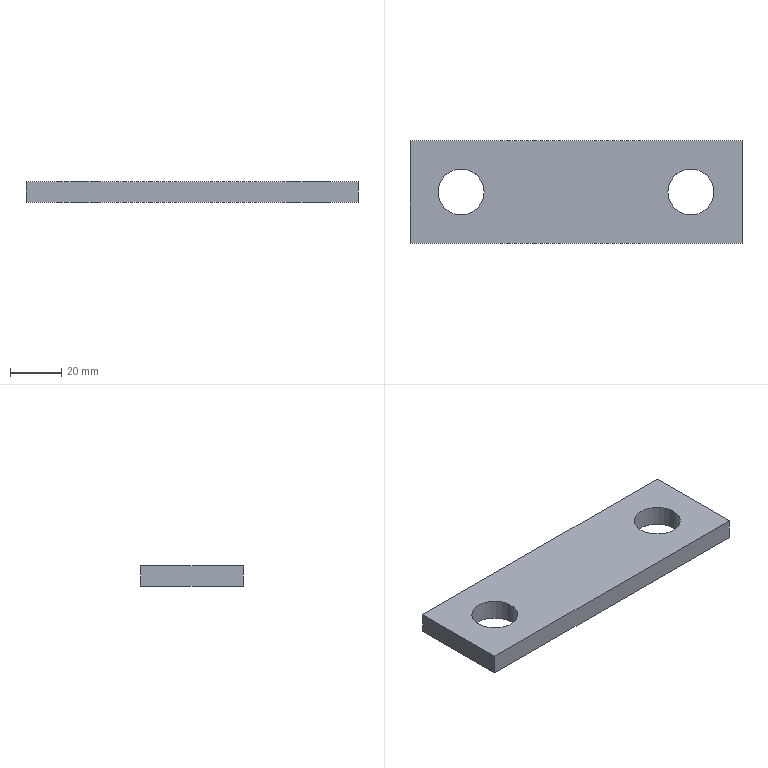Part | STEP file | JBZQ4348-1997 shaft end baffle 60 | 1 solid | 10 faces | box 130 x 40 x 8 mm | volume 37528 mm3 | plane 6 | cylinder 4 | commonest cylinder face diameters 18 x4
STEP:
#1=CARTESIAN_POINT('',(0.,0.,0.));
#2=DIRECTION('',(0.,0.,1.));
#3=DIRECTION('',(1.,0.,0.));
#4=AXIS2_PLACEMENT_3D('',#1,#2,#3);
#5=CARTESIAN_POINT('',(36.,0.,8.));
#6=VERTEX_POINT('',#5);
#7=CARTESIAN_POINT('',(36.,0.,0.));
#8=VERTEX_POINT('',#7);
#9=CARTESIAN_POINT('',(36.,0.,8.));
#10=DIRECTION('',(0.,0.,-1.));
#11=VECTOR('',#10,1.);
#12=LINE('',#9,#11);
#13=CARTESIAN_POINT('',(45.,0.,8.));
#14=DIRECTION('',(0.,0.,-1.));
#15=DIRECTION('',(-1.,0.,0.));
#16=AXIS2_PLACEMENT_3D('',#13,#14,#15);
#17=CYLINDRICAL_SURFACE('',#16,9.);
#18=CARTESIAN_POINT('',(6.283,0.));
#19=DIRECTION('',(0.,1.));
#20=VECTOR('',#19,1.);
#21=LINE('',#18,#20);
#22=(GEOMETRIC_REPRESENTATION_CONTEXT(2)PARAMETRIC_REPRESENTATION_CONTEXT()REPRESENTATION_CONTEXT('',''));
#23=DEFINITIONAL_REPRESENTATION('',(#21),#22);
#24=PCURVE('',#17,#23);
#25=CARTESIAN_POINT('',(45.,0.,8.));
#26=DIRECTION('',(0.,0.,-1.));
#27=DIRECTION('',(-1.,0.,0.));
#28=AXIS2_PLACEMENT_3D('',#25,#26,#27);
#29=CYLINDRICAL_SURFACE('',#28,9.);
#30=CARTESIAN_POINT('',(0.,0.));
#31=DIRECTION('',(0.,1.));
#32=VECTOR('',#31,1.);
#33=LINE('',#30,#32);
#34=(GEOMETRIC_REPRESENTATION_CONTEXT(2)PARAMETRIC_REPRESENTATION_CONTEXT()REPRESENTATION_CONTEXT('',''));
#35=DEFINITIONAL_REPRESENTATION('',(#33),#34);
#36=PCURVE('',#29,#35);
#37=SURFACE_CURVE('',#12,(#24,#36),.PCURVE_S1.);
#38=EDGE_CURVE('',#6,#8,#37,.T.);
#39=ORIENTED_EDGE('',*,*,#38,.T.);
#40=CARTESIAN_POINT('',(54.,0.,0.));
#41=VERTEX_POINT('',#40);
#42=CARTESIAN_POINT('',(45.,0.,0.));
#43=DIRECTION('',(0.,0.,1.));
#44=DIRECTION('',(1.,0.,0.));
#45=AXIS2_PLACEMENT_3D('',#42,#43,#44);
#46=CIRCLE('',#45,9.);
#47=CARTESIAN_POINT('',(9.425,8.));
#48=DIRECTION('',(-1.,0.));
#49=VECTOR('',#48,1.);
#50=LINE('',#47,#49);
#51=(GEOMETRIC_REPRESENTATION_CONTEXT(2)PARAMETRIC_REPRESENTATION_CONTEXT()REPRESENTATION_CONTEXT('',''));
#52=DEFINITIONAL_REPRESENTATION('',(#50),#51);
#53=PCURVE('',#17,#52);
#54=CARTESIAN_POINT('',(-65.,20.,0.));
#55=DIRECTION('',(0.,0.,1.));
#56=DIRECTION('',(1.,0.,0.));
#57=AXIS2_PLACEMENT_3D('',#54,#55,#56);
#58=PLANE('',#57);
#59=CARTESIAN_POINT('',(110.,-20.));
#60=DIRECTION('',(1.,0.));
#61=AXIS2_PLACEMENT_2D('',#59,#60);
#62=CIRCLE('',#61,9.);
#63=(GEOMETRIC_REPRESENTATION_CONTEXT(2)PARAMETRIC_REPRESENTATION_CONTEXT()REPRESENTATION_CONTEXT('',''));
#64=DEFINITIONAL_REPRESENTATION('',(#62),#63);
#65=PCURVE('',#58,#64);
#66=SURFACE_CURVE('',#46,(#53,#65),.PCURVE_S1.);
#67=EDGE_CURVE('',#8,#41,#66,.T.);
#68=ORIENTED_EDGE('',*,*,#67,.T.);
#69=CARTESIAN_POINT('',(54.,0.,8.));
#70=VERTEX_POINT('',#69);
#71=CARTESIAN_POINT('',(54.,0.,8.));
#72=DIRECTION('',(0.,0.,-1.));
#73=VECTOR('',#72,1.);
#74=LINE('',#71,#73);
#75=CARTESIAN_POINT('',(3.142,0.));
#76=DIRECTION('',(0.,1.));
#77=VECTOR('',#76,1.);
#78=LINE('',#75,#77);
#79=(GEOMETRIC_REPRESENTATION_CONTEXT(2)PARAMETRIC_REPRESENTATION_CONTEXT()REPRESENTATION_CONTEXT('',''));
#80=DEFINITIONAL_REPRESENTATION('',(#78),#79);
#81=PCURVE('',#17,#80);
#82=CARTESIAN_POINT('',(3.142,0.));
#83=DIRECTION('',(0.,1.));
#84=VECTOR('',#83,1.);
#85=LINE('',#82,#84);
#86=(GEOMETRIC_REPRESENTATION_CONTEXT(2)PARAMETRIC_REPRESENTATION_CONTEXT()REPRESENTATION_CONTEXT('',''));
#87=DEFINITIONAL_REPRESENTATION('',(#85),#86);
#88=PCURVE('',#29,#87);
#89=SURFACE_CURVE('',#74,(#81,#88),.PCURVE_S1.);
#90=EDGE_CURVE('',#70,#41,#89,.T.);
#91=ORIENTED_EDGE('',*,*,#90,.F.);
#92=CARTESIAN_POINT('',(45.,0.,8.));
#93=DIRECTION('',(0.,0.,1.));
#94=DIRECTION('',(1.,0.,0.));
#95=AXIS2_PLACEMENT_3D('',#92,#93,#94);
#96=CIRCLE('',#95,9.);
#97=CARTESIAN_POINT('',(9.425,0.));
#98=DIRECTION('',(-1.,0.));
#99=VECTOR('',#98,1.);
#100=LINE('',#97,#99);
#101=(GEOMETRIC_REPRESENTATION_CONTEXT(2)PARAMETRIC_REPRESENTATION_CONTEXT()REPRESENTATION_CONTEXT('',''));
#102=DEFINITIONAL_REPRESENTATION('',(#100),#101);
#103=PCURVE('',#17,#102);
#104=CARTESIAN_POINT('',(-65.,20.,8.));
#105=DIRECTION('',(0.,0.,1.));
#106=DIRECTION('',(1.,0.,0.));
#107=AXIS2_PLACEMENT_3D('',#104,#105,#106);
#108=PLANE('',#107);
#109=CARTESIAN_POINT('',(110.,-20.));
#110=DIRECTION('',(1.,0.));
#111=AXIS2_PLACEMENT_2D('',#109,#110);
#112=CIRCLE('',#111,9.);
#113=(GEOMETRIC_REPRESENTATION_CONTEXT(2)PARAMETRIC_REPRESENTATION_CONTEXT()REPRESENTATION_CONTEXT('',''));
#114=DEFINITIONAL_REPRESENTATION('',(#112),#113);
#115=PCURVE('',#108,#114);
#116=SURFACE_CURVE('',#96,(#103,#115),.PCURVE_S1.);
#117=EDGE_CURVE('',#6,#70,#116,.T.);
#118=ORIENTED_EDGE('',*,*,#117,.F.);
#119=EDGE_LOOP('',(#39,#68,#91,#118));
#120=FACE_BOUND('',#119,.F.);
#121=ADVANCED_FACE('',(#120),#17,.F.);
#122=CARTESIAN_POINT('',(-54.,0.,8.));
#123=VERTEX_POINT('',#122);
#124=CARTESIAN_POINT('',(-54.,0.,0.));
#125=VERTEX_POINT('',#124);
#126=CARTESIAN_POINT('',(-54.,0.,8.));
#127=DIRECTION('',(0.,0.,-1.));
#128=VECTOR('',#127,1.);
#129=LINE('',#126,#128);
#130=CARTESIAN_POINT('',(-45.,0.,8.));
#131=DIRECTION('',(0.,0.,-1.));
#132=DIRECTION('',(-1.,0.,0.));
#133=AXIS2_PLACEMENT_3D('',#130,#131,#132);
#134=CYLINDRICAL_SURFACE('',#133,9.);
#135=CARTESIAN_POINT('',(6.283,0.));
#136=DIRECTION('',(0.,1.));
#137=VECTOR('',#136,1.);
#138=LINE('',#135,#137);
#139=(GEOMETRIC_REPRESENTATION_CONTEXT(2)PARAMETRIC_REPRESENTATION_CONTEXT()REPRESENTATION_CONTEXT('',''));
#140=DEFINITIONAL_REPRESENTATION('',(#138),#139);
#141=PCURVE('',#134,#140);
#142=CARTESIAN_POINT('',(-45.,0.,8.));
#143=DIRECTION('',(0.,0.,-1.));
#144=DIRECTION('',(-1.,0.,0.));
#145=AXIS2_PLACEMENT_3D('',#142,#143,#144);
#146=CYLINDRICAL_SURFACE('',#145,9.);
#147=CARTESIAN_POINT('',(0.,0.));
#148=DIRECTION('',(0.,1.));
#149=VECTOR('',#148,1.);
#150=LINE('',#147,#149);
#151=(GEOMETRIC_REPRESENTATION_CONTEXT(2)PARAMETRIC_REPRESENTATION_CONTEXT()REPRESENTATION_CONTEXT('',''));
#152=DEFINITIONAL_REPRESENTATION('',(#150),#151);
#153=PCURVE('',#146,#152);
#154=SURFACE_CURVE('',#129,(#141,#153),.PCURVE_S1.);
#155=EDGE_CURVE('',#123,#125,#154,.T.);
#156=ORIENTED_EDGE('',*,*,#155,.T.);
#157=CARTESIAN_POINT('',(-36.,0.,0.));
#158=VERTEX_POINT('',#157);
#159=CARTESIAN_POINT('',(-45.,0.,0.));
#160=DIRECTION('',(0.,0.,1.));
#161=DIRECTION('',(1.,0.,0.));
#162=AXIS2_PLACEMENT_3D('',#159,#160,#161);
#163=CIRCLE('',#162,9.);
#164=CARTESIAN_POINT('',(9.425,8.));
#165=DIRECTION('',(-1.,0.));
#166=VECTOR('',#165,1.);
#167=LINE('',#164,#166);
#168=(GEOMETRIC_REPRESENTATION_CONTEXT(2)PARAMETRIC_REPRESENTATION_CONTEXT()REPRESENTATION_CONTEXT('',''));
#169=DEFINITIONAL_REPRESENTATION('',(#167),#168);
#170=PCURVE('',#134,#169);
#171=CARTESIAN_POINT('',(20.,-20.));
#172=DIRECTION('',(1.,0.));
#173=AXIS2_PLACEMENT_2D('',#171,#172);
#174=CIRCLE('',#173,9.);
#175=(GEOMETRIC_REPRESENTATION_CONTEXT(2)PARAMETRIC_REPRESENTATION_CONTEXT()REPRESENTATION_CONTEXT('',''));
#176=DEFINITIONAL_REPRESENTATION('',(#174),#175);
#177=PCURVE('',#58,#176);
#178=SURFACE_CURVE('',#163,(#170,#177),.PCURVE_S1.);
#179=EDGE_CURVE('',#125,#158,#178,.T.);
#180=ORIENTED_EDGE('',*,*,#179,.T.);
#181=CARTESIAN_POINT('',(-36.,0.,8.));
#182=VERTEX_POINT('',#181);
#183=CARTESIAN_POINT('',(-36.,0.,8.));
#184=DIRECTION('',(0.,0.,-1.));
#185=VECTOR('',#184,1.);
#186=LINE('',#183,#185);
#187=CARTESIAN_POINT('',(3.142,0.));
#188=DIRECTION('',(0.,1.));
#189=VECTOR('',#188,1.);
#190=LINE('',#187,#189);
#191=(GEOMETRIC_REPRESENTATION_CONTEXT(2)PARAMETRIC_REPRESENTATION_CONTEXT()REPRESENTATION_CONTEXT('',''));
#192=DEFINITIONAL_REPRESENTATION('',(#190),#191);
#193=PCURVE('',#134,#192);
#194=CARTESIAN_POINT('',(3.142,0.));
#195=DIRECTION('',(0.,1.));
#196=VECTOR('',#195,1.);
#197=LINE('',#194,#196);
#198=(GEOMETRIC_REPRESENTATION_CONTEXT(2)PARAMETRIC_REPRESENTATION_CONTEXT()REPRESENTATION_CONTEXT('',''));
#199=DEFINITIONAL_REPRESENTATION('',(#197),#198);
#200=PCURVE('',#146,#199);
#201=SURFACE_CURVE('',#186,(#193,#200),.PCURVE_S1.);
#202=EDGE_CURVE('',#182,#158,#201,.T.);
#203=ORIENTED_EDGE('',*,*,#202,.F.);
#204=CARTESIAN_POINT('',(-45.,0.,8.));
#205=DIRECTION('',(0.,0.,1.));
#206=DIRECTION('',(1.,0.,0.));
#207=AXIS2_PLACEMENT_3D('',#204,#205,#206);
#208=CIRCLE('',#207,9.);
#209=CARTESIAN_POINT('',(9.425,0.));
#210=DIRECTION('',(-1.,0.));
#211=VECTOR('',#210,1.);
#212=LINE('',#209,#211);
#213=(GEOMETRIC_REPRESENTATION_CONTEXT(2)PARAMETRIC_REPRESENTATION_CONTEXT()REPRESENTATION_CONTEXT('',''));
#214=DEFINITIONAL_REPRESENTATION('',(#212),#213);
#215=PCURVE('',#134,#214);
#216=CARTESIAN_POINT('',(20.,-20.));
#217=DIRECTION('',(1.,0.));
#218=AXIS2_PLACEMENT_2D('',#216,#217);
#219=CIRCLE('',#218,9.);
#220=(GEOMETRIC_REPRESENTATION_CONTEXT(2)PARAMETRIC_REPRESENTATION_CONTEXT()REPRESENTATION_CONTEXT('',''));
#221=DEFINITIONAL_REPRESENTATION('',(#219),#220);
#222=PCURVE('',#108,#221);
#223=SURFACE_CURVE('',#208,(#215,#222),.PCURVE_S1.);
#224=EDGE_CURVE('',#123,#182,#223,.T.);
#225=ORIENTED_EDGE('',*,*,#224,.F.);
#226=EDGE_LOOP('',(#156,#180,#203,#225));
#227=FACE_BOUND('',#226,.F.);
#228=ADVANCED_FACE('',(#227),#134,.F.);
#229=ORIENTED_EDGE('',*,*,#224,.F.);
#230=CARTESIAN_POINT('',(-45.,0.,8.));
#231=DIRECTION('',(0.,0.,1.));
#232=DIRECTION('',(1.,0.,0.));
#233=AXIS2_PLACEMENT_3D('',#230,#231,#232);
#234=CIRCLE('',#233,9.);
#235=CARTESIAN_POINT('',(20.,-20.));
#236=DIRECTION('',(1.,0.));
#237=AXIS2_PLACEMENT_2D('',#235,#236);
#238=CIRCLE('',#237,9.);
#239=(GEOMETRIC_REPRESENTATION_CONTEXT(2)PARAMETRIC_REPRESENTATION_CONTEXT()REPRESENTATION_CONTEXT('',''));
#240=DEFINITIONAL_REPRESENTATION('',(#238),#239);
#241=PCURVE('',#108,#240);
#242=CARTESIAN_POINT('',(3.142,0.));
#243=DIRECTION('',(-1.,0.));
#244=VECTOR('',#243,1.);
#245=LINE('',#242,#244);
#246=(GEOMETRIC_REPRESENTATION_CONTEXT(2)PARAMETRIC_REPRESENTATION_CONTEXT()REPRESENTATION_CONTEXT('',''));
#247=DEFINITIONAL_REPRESENTATION('',(#245),#246);
#248=PCURVE('',#146,#247);
#249=SURFACE_CURVE('',#234,(#241,#248),.PCURVE_S1.);
#250=EDGE_CURVE('',#182,#123,#249,.T.);
#251=ORIENTED_EDGE('',*,*,#250,.F.);
#252=EDGE_LOOP('',(#229,#251));
#253=FACE_BOUND('',#252,.T.);
#254=CARTESIAN_POINT('',(65.,20.,8.));
#255=VERTEX_POINT('',#254);
#256=CARTESIAN_POINT('',(-65.,20.,8.));
#257=VERTEX_POINT('',#256);
#258=CARTESIAN_POINT('',(65.,20.,8.));
#259=DIRECTION('',(-1.,0.,0.));
#260=VECTOR('',#259,1.);
#261=LINE('',#258,#260);
#262=CARTESIAN_POINT('',(130.,0.));
#263=DIRECTION('',(-1.,0.));
#264=VECTOR('',#263,1.);
#265=LINE('',#262,#264);
#266=(GEOMETRIC_REPRESENTATION_CONTEXT(2)PARAMETRIC_REPRESENTATION_CONTEXT()REPRESENTATION_CONTEXT('',''));
#267=DEFINITIONAL_REPRESENTATION('',(#265),#266);
#268=PCURVE('',#108,#267);
#269=CARTESIAN_POINT('',(65.,20.,8.));
#270=DIRECTION('',(0.,-1.,0.));
#271=DIRECTION('',(1.,0.,0.));
#272=AXIS2_PLACEMENT_3D('',#269,#270,#271);
#273=PLANE('',#272);
#274=CARTESIAN_POINT('',(0.,0.));
#275=DIRECTION('',(-1.,0.));
#276=VECTOR('',#275,1.);
#277=LINE('',#274,#276);
#278=(GEOMETRIC_REPRESENTATION_CONTEXT(2)PARAMETRIC_REPRESENTATION_CONTEXT()REPRESENTATION_CONTEXT('',''));
#279=DEFINITIONAL_REPRESENTATION('',(#277),#278);
#280=PCURVE('',#273,#279);
#281=SURFACE_CURVE('',#261,(#268,#280),.PCURVE_S1.);
#282=EDGE_CURVE('',#255,#257,#281,.T.);
#283=ORIENTED_EDGE('',*,*,#282,.T.);
#284=CARTESIAN_POINT('',(-65.,-20.,8.));
#285=VERTEX_POINT('',#284);
#286=CARTESIAN_POINT('',(-65.,20.,8.));
#287=DIRECTION('',(0.,-1.,0.));
#288=VECTOR('',#287,1.);
#289=LINE('',#286,#288);
#290=CARTESIAN_POINT('',(0.,0.));
#291=DIRECTION('',(0.,-1.));
#292=VECTOR('',#291,1.);
#293=LINE('',#290,#292);
#294=(GEOMETRIC_REPRESENTATION_CONTEXT(2)PARAMETRIC_REPRESENTATION_CONTEXT()REPRESENTATION_CONTEXT('',''));
#295=DEFINITIONAL_REPRESENTATION('',(#293),#294);
#296=PCURVE('',#108,#295);
#297=CARTESIAN_POINT('',(-65.,20.,8.));
#298=DIRECTION('',(1.,0.,0.));
#299=DIRECTION('',(0.,0.,-1.));
#300=AXIS2_PLACEMENT_3D('',#297,#298,#299);
#301=PLANE('',#300);
#302=CARTESIAN_POINT('',(0.,0.));
#303=DIRECTION('',(0.,-1.));
#304=VECTOR('',#303,1.);
#305=LINE('',#302,#304);
#306=(GEOMETRIC_REPRESENTATION_CONTEXT(2)PARAMETRIC_REPRESENTATION_CONTEXT()REPRESENTATION_CONTEXT('',''));
#307=DEFINITIONAL_REPRESENTATION('',(#305),#306);
#308=PCURVE('',#301,#307);
#309=SURFACE_CURVE('',#289,(#296,#308),.PCURVE_S1.);
#310=EDGE_CURVE('',#257,#285,#309,.T.);
#311=ORIENTED_EDGE('',*,*,#310,.T.);
#312=CARTESIAN_POINT('',(65.,-20.,8.));
#313=VERTEX_POINT('',#312);
#314=CARTESIAN_POINT('',(-65.,-20.,8.));
#315=DIRECTION('',(1.,0.,0.));
#316=VECTOR('',#315,1.);
#317=LINE('',#314,#316);
#318=CARTESIAN_POINT('',(0.,-40.));
#319=DIRECTION('',(1.,0.));
#320=VECTOR('',#319,1.);
#321=LINE('',#318,#320);
#322=(GEOMETRIC_REPRESENTATION_CONTEXT(2)PARAMETRIC_REPRESENTATION_CONTEXT()REPRESENTATION_CONTEXT('',''));
#323=DEFINITIONAL_REPRESENTATION('',(#321),#322);
#324=PCURVE('',#108,#323);
#325=CARTESIAN_POINT('',(-65.,-20.,8.));
#326=DIRECTION('',(0.,1.,0.));
#327=DIRECTION('',(0.,0.,1.));
#328=AXIS2_PLACEMENT_3D('',#325,#326,#327);
#329=PLANE('',#328);
#330=CARTESIAN_POINT('',(0.,0.));
#331=DIRECTION('',(0.,1.));
#332=VECTOR('',#331,1.);
#333=LINE('',#330,#332);
#334=(GEOMETRIC_REPRESENTATION_CONTEXT(2)PARAMETRIC_REPRESENTATION_CONTEXT()REPRESENTATION_CONTEXT('',''));
#335=DEFINITIONAL_REPRESENTATION('',(#333),#334);
#336=PCURVE('',#329,#335);
#337=SURFACE_CURVE('',#317,(#324,#336),.PCURVE_S1.);
#338=EDGE_CURVE('',#285,#313,#337,.T.);
#339=ORIENTED_EDGE('',*,*,#338,.T.);
#340=CARTESIAN_POINT('',(65.,-20.,8.));
#341=DIRECTION('',(0.,1.,0.));
#342=VECTOR('',#341,1.);
#343=LINE('',#340,#342);
#344=CARTESIAN_POINT('',(130.,-40.));
#345=DIRECTION('',(0.,1.));
#346=VECTOR('',#345,1.);
#347=LINE('',#344,#346);
#348=(GEOMETRIC_REPRESENTATION_CONTEXT(2)PARAMETRIC_REPRESENTATION_CONTEXT()REPRESENTATION_CONTEXT('',''));
#349=DEFINITIONAL_REPRESENTATION('',(#347),#348);
#350=PCURVE('',#108,#349);
#351=CARTESIAN_POINT('',(65.,-20.,8.));
#352=DIRECTION('',(-1.,0.,0.));
#353=DIRECTION('',(0.,0.,1.));
#354=AXIS2_PLACEMENT_3D('',#351,#352,#353);
#355=PLANE('',#354);
#356=CARTESIAN_POINT('',(0.,0.));
#357=DIRECTION('',(0.,1.));
#358=VECTOR('',#357,1.);
#359=LINE('',#356,#358);
#360=(GEOMETRIC_REPRESENTATION_CONTEXT(2)PARAMETRIC_REPRESENTATION_CONTEXT()REPRESENTATION_CONTEXT('',''));
#361=DEFINITIONAL_REPRESENTATION('',(#359),#360);
#362=PCURVE('',#355,#361);
#363=SURFACE_CURVE('',#343,(#350,#362),.PCURVE_S1.);
#364=EDGE_CURVE('',#313,#255,#363,.T.);
#365=ORIENTED_EDGE('',*,*,#364,.T.);
#366=EDGE_LOOP('',(#283,#311,#339,#365));
#367=FACE_BOUND('',#366,.T.);
#368=ORIENTED_EDGE('',*,*,#117,.F.);
#369=CARTESIAN_POINT('',(45.,0.,8.));
#370=DIRECTION('',(0.,0.,1.));
#371=DIRECTION('',(1.,0.,0.));
#372=AXIS2_PLACEMENT_3D('',#369,#370,#371);
#373=CIRCLE('',#372,9.);
#374=CARTESIAN_POINT('',(110.,-20.));
#375=DIRECTION('',(1.,0.));
#376=AXIS2_PLACEMENT_2D('',#374,#375);
#377=CIRCLE('',#376,9.);
#378=(GEOMETRIC_REPRESENTATION_CONTEXT(2)PARAMETRIC_REPRESENTATION_CONTEXT()REPRESENTATION_CONTEXT('',''));
#379=DEFINITIONAL_REPRESENTATION('',(#377),#378);
#380=PCURVE('',#108,#379);
#381=CARTESIAN_POINT('',(3.142,0.));
#382=DIRECTION('',(-1.,0.));
#383=VECTOR('',#382,1.);
#384=LINE('',#381,#383);
#385=(GEOMETRIC_REPRESENTATION_CONTEXT(2)PARAMETRIC_REPRESENTATION_CONTEXT()REPRESENTATION_CONTEXT('',''));
#386=DEFINITIONAL_REPRESENTATION('',(#384),#385);
#387=PCURVE('',#29,#386);
#388=SURFACE_CURVE('',#373,(#380,#387),.PCURVE_S1.);
#389=EDGE_CURVE('',#70,#6,#388,.T.);
#390=ORIENTED_EDGE('',*,*,#389,.F.);
#391=EDGE_LOOP('',(#368,#390));
#392=FACE_BOUND('',#391,.T.);
#393=ADVANCED_FACE('',(#253,#367,#392),#108,.T.);
#394=ORIENTED_EDGE('',*,*,#179,.T.);
#395=CARTESIAN_POINT('',(-45.,0.,0.));
#396=DIRECTION('',(0.,0.,1.));
#397=DIRECTION('',(1.,0.,0.));
#398=AXIS2_PLACEMENT_3D('',#395,#396,#397);
#399=CIRCLE('',#398,9.);
#400=CARTESIAN_POINT('',(20.,-20.));
#401=DIRECTION('',(1.,0.));
#402=AXIS2_PLACEMENT_2D('',#400,#401);
#403=CIRCLE('',#402,9.);
#404=(GEOMETRIC_REPRESENTATION_CONTEXT(2)PARAMETRIC_REPRESENTATION_CONTEXT()REPRESENTATION_CONTEXT('',''));
#405=DEFINITIONAL_REPRESENTATION('',(#403),#404);
#406=PCURVE('',#58,#405);
#407=CARTESIAN_POINT('',(3.142,8.));
#408=DIRECTION('',(-1.,0.));
#409=VECTOR('',#408,1.);
#410=LINE('',#407,#409);
#411=(GEOMETRIC_REPRESENTATION_CONTEXT(2)PARAMETRIC_REPRESENTATION_CONTEXT()REPRESENTATION_CONTEXT('',''));
#412=DEFINITIONAL_REPRESENTATION('',(#410),#411);
#413=PCURVE('',#146,#412);
#414=SURFACE_CURVE('',#399,(#406,#413),.PCURVE_S1.);
#415=EDGE_CURVE('',#158,#125,#414,.T.);
#416=ORIENTED_EDGE('',*,*,#415,.T.);
#417=EDGE_LOOP('',(#394,#416));
#418=FACE_BOUND('',#417,.T.);
#419=CARTESIAN_POINT('',(65.,20.,0.));
#420=VERTEX_POINT('',#419);
#421=CARTESIAN_POINT('',(-65.,20.,0.));
#422=VERTEX_POINT('',#421);
#423=CARTESIAN_POINT('',(65.,20.,0.));
#424=DIRECTION('',(-1.,0.,0.));
#425=VECTOR('',#424,1.);
#426=LINE('',#423,#425);
#427=CARTESIAN_POINT('',(130.,0.));
#428=DIRECTION('',(-1.,0.));
#429=VECTOR('',#428,1.);
#430=LINE('',#427,#429);
#431=(GEOMETRIC_REPRESENTATION_CONTEXT(2)PARAMETRIC_REPRESENTATION_CONTEXT()REPRESENTATION_CONTEXT('',''));
#432=DEFINITIONAL_REPRESENTATION('',(#430),#431);
#433=PCURVE('',#58,#432);
#434=CARTESIAN_POINT('',(0.,-8.));
#435=DIRECTION('',(-1.,0.));
#436=VECTOR('',#435,1.);
#437=LINE('',#434,#436);
#438=(GEOMETRIC_REPRESENTATION_CONTEXT(2)PARAMETRIC_REPRESENTATION_CONTEXT()REPRESENTATION_CONTEXT('',''));
#439=DEFINITIONAL_REPRESENTATION('',(#437),#438);
#440=PCURVE('',#273,#439);
#441=SURFACE_CURVE('',#426,(#433,#440),.PCURVE_S1.);
#442=EDGE_CURVE('',#420,#422,#441,.T.);
#443=ORIENTED_EDGE('',*,*,#442,.F.);
#444=CARTESIAN_POINT('',(65.,-20.,0.));
#445=VERTEX_POINT('',#444);
#446=CARTESIAN_POINT('',(65.,-20.,0.));
#447=DIRECTION('',(0.,1.,0.));
#448=VECTOR('',#447,1.);
#449=LINE('',#446,#448);
#450=CARTESIAN_POINT('',(130.,-40.));
#451=DIRECTION('',(0.,1.));
#452=VECTOR('',#451,1.);
#453=LINE('',#450,#452);
#454=(GEOMETRIC_REPRESENTATION_CONTEXT(2)PARAMETRIC_REPRESENTATION_CONTEXT()REPRESENTATION_CONTEXT('',''));
#455=DEFINITIONAL_REPRESENTATION('',(#453),#454);
#456=PCURVE('',#58,#455);
#457=CARTESIAN_POINT('',(-8.,0.));
#458=DIRECTION('',(0.,1.));
#459=VECTOR('',#458,1.);
#460=LINE('',#457,#459);
#461=(GEOMETRIC_REPRESENTATION_CONTEXT(2)PARAMETRIC_REPRESENTATION_CONTEXT()REPRESENTATION_CONTEXT('',''));
#462=DEFINITIONAL_REPRESENTATION('',(#460),#461);
#463=PCURVE('',#355,#462);
#464=SURFACE_CURVE('',#449,(#456,#463),.PCURVE_S1.);
#465=EDGE_CURVE('',#445,#420,#464,.T.);
#466=ORIENTED_EDGE('',*,*,#465,.F.);
#467=CARTESIAN_POINT('',(-65.,-20.,0.));
#468=VERTEX_POINT('',#467);
#469=CARTESIAN_POINT('',(-65.,-20.,0.));
#470=DIRECTION('',(1.,0.,0.));
#471=VECTOR('',#470,1.);
#472=LINE('',#469,#471);
#473=CARTESIAN_POINT('',(0.,-40.));
#474=DIRECTION('',(1.,0.));
#475=VECTOR('',#474,1.);
#476=LINE('',#473,#475);
#477=(GEOMETRIC_REPRESENTATION_CONTEXT(2)PARAMETRIC_REPRESENTATION_CONTEXT()REPRESENTATION_CONTEXT('',''));
#478=DEFINITIONAL_REPRESENTATION('',(#476),#477);
#479=PCURVE('',#58,#478);
#480=CARTESIAN_POINT('',(-8.,0.));
#481=DIRECTION('',(0.,1.));
#482=VECTOR('',#481,1.);
#483=LINE('',#480,#482);
#484=(GEOMETRIC_REPRESENTATION_CONTEXT(2)PARAMETRIC_REPRESENTATION_CONTEXT()REPRESENTATION_CONTEXT('',''));
#485=DEFINITIONAL_REPRESENTATION('',(#483),#484);
#486=PCURVE('',#329,#485);
#487=SURFACE_CURVE('',#472,(#479,#486),.PCURVE_S1.);
#488=EDGE_CURVE('',#468,#445,#487,.T.);
#489=ORIENTED_EDGE('',*,*,#488,.F.);
#490=CARTESIAN_POINT('',(-65.,20.,0.));
#491=DIRECTION('',(0.,-1.,0.));
#492=VECTOR('',#491,1.);
#493=LINE('',#490,#492);
#494=CARTESIAN_POINT('',(0.,0.));
#495=DIRECTION('',(0.,-1.));
#496=VECTOR('',#495,1.);
#497=LINE('',#494,#496);
#498=(GEOMETRIC_REPRESENTATION_CONTEXT(2)PARAMETRIC_REPRESENTATION_CONTEXT()REPRESENTATION_CONTEXT('',''));
#499=DEFINITIONAL_REPRESENTATION('',(#497),#498);
#500=PCURVE('',#58,#499);
#501=CARTESIAN_POINT('',(8.,0.));
#502=DIRECTION('',(0.,-1.));
#503=VECTOR('',#502,1.);
#504=LINE('',#501,#503);
#505=(GEOMETRIC_REPRESENTATION_CONTEXT(2)PARAMETRIC_REPRESENTATION_CONTEXT()REPRESENTATION_CONTEXT('',''));
#506=DEFINITIONAL_REPRESENTATION('',(#504),#505);
#507=PCURVE('',#301,#506);
#508=SURFACE_CURVE('',#493,(#500,#507),.PCURVE_S1.);
#509=EDGE_CURVE('',#422,#468,#508,.T.);
#510=ORIENTED_EDGE('',*,*,#509,.F.);
#511=EDGE_LOOP('',(#443,#466,#489,#510));
#512=FACE_BOUND('',#511,.T.);
#513=ORIENTED_EDGE('',*,*,#67,.T.);
#514=CARTESIAN_POINT('',(45.,0.,0.));
#515=DIRECTION('',(0.,0.,1.));
#516=DIRECTION('',(1.,0.,0.));
#517=AXIS2_PLACEMENT_3D('',#514,#515,#516);
#518=CIRCLE('',#517,9.);
#519=CARTESIAN_POINT('',(110.,-20.));
#520=DIRECTION('',(1.,0.));
#521=AXIS2_PLACEMENT_2D('',#519,#520);
#522=CIRCLE('',#521,9.);
#523=(GEOMETRIC_REPRESENTATION_CONTEXT(2)PARAMETRIC_REPRESENTATION_CONTEXT()REPRESENTATION_CONTEXT('',''));
#524=DEFINITIONAL_REPRESENTATION('',(#522),#523);
#525=PCURVE('',#58,#524);
#526=CARTESIAN_POINT('',(3.142,8.));
#527=DIRECTION('',(-1.,0.));
#528=VECTOR('',#527,1.);
#529=LINE('',#526,#528);
#530=(GEOMETRIC_REPRESENTATION_CONTEXT(2)PARAMETRIC_REPRESENTATION_CONTEXT()REPRESENTATION_CONTEXT('',''));
#531=DEFINITIONAL_REPRESENTATION('',(#529),#530);
#532=PCURVE('',#29,#531);
#533=SURFACE_CURVE('',#518,(#525,#532),.PCURVE_S1.);
#534=EDGE_CURVE('',#41,#8,#533,.T.);
#535=ORIENTED_EDGE('',*,*,#534,.T.);
#536=EDGE_LOOP('',(#513,#535));
#537=FACE_BOUND('',#536,.T.);
#538=ADVANCED_FACE('',(#418,#512,#537),#58,.F.);
#539=ORIENTED_EDGE('',*,*,#442,.T.);
#540=CARTESIAN_POINT('',(-65.,20.,8.));
#541=DIRECTION('',(0.,0.,-1.));
#542=VECTOR('',#541,1.);
#543=LINE('',#540,#542);
#544=CARTESIAN_POINT('',(-130.,0.));
#545=DIRECTION('',(0.,-1.));
#546=VECTOR('',#545,1.);
#547=LINE('',#544,#546);
#548=(GEOMETRIC_REPRESENTATION_CONTEXT(2)PARAMETRIC_REPRESENTATION_CONTEXT()REPRESENTATION_CONTEXT('',''));
#549=DEFINITIONAL_REPRESENTATION('',(#547),#548);
#550=PCURVE('',#273,#549);
#551=CARTESIAN_POINT('',(0.,0.));
#552=DIRECTION('',(1.,0.));
#553=VECTOR('',#552,1.);
#554=LINE('',#551,#553);
#555=(GEOMETRIC_REPRESENTATION_CONTEXT(2)PARAMETRIC_REPRESENTATION_CONTEXT()REPRESENTATION_CONTEXT('',''));
#556=DEFINITIONAL_REPRESENTATION('',(#554),#555);
#557=PCURVE('',#301,#556);
#558=SURFACE_CURVE('',#543,(#550,#557),.PCURVE_S1.);
#559=EDGE_CURVE('',#257,#422,#558,.T.);
#560=ORIENTED_EDGE('',*,*,#559,.F.);
#561=ORIENTED_EDGE('',*,*,#282,.F.);
#562=CARTESIAN_POINT('',(65.,20.,8.));
#563=DIRECTION('',(0.,0.,-1.));
#564=VECTOR('',#563,1.);
#565=LINE('',#562,#564);
#566=CARTESIAN_POINT('',(0.,0.));
#567=DIRECTION('',(0.,-1.));
#568=VECTOR('',#567,1.);
#569=LINE('',#566,#568);
#570=(GEOMETRIC_REPRESENTATION_CONTEXT(2)PARAMETRIC_REPRESENTATION_CONTEXT()REPRESENTATION_CONTEXT('',''));
#571=DEFINITIONAL_REPRESENTATION('',(#569),#570);
#572=PCURVE('',#273,#571);
#573=CARTESIAN_POINT('',(0.,40.));
#574=DIRECTION('',(-1.,0.));
#575=VECTOR('',#574,1.);
#576=LINE('',#573,#575);
#577=(GEOMETRIC_REPRESENTATION_CONTEXT(2)PARAMETRIC_REPRESENTATION_CONTEXT()REPRESENTATION_CONTEXT('',''));
#578=DEFINITIONAL_REPRESENTATION('',(#576),#577);
#579=PCURVE('',#355,#578);
#580=SURFACE_CURVE('',#565,(#572,#579),.PCURVE_S1.);
#581=EDGE_CURVE('',#255,#420,#580,.T.);
#582=ORIENTED_EDGE('',*,*,#581,.T.);
#583=EDGE_LOOP('',(#539,#560,#561,#582));
#584=FACE_BOUND('',#583,.T.);
#585=ADVANCED_FACE('',(#584),#273,.F.);
#586=ORIENTED_EDGE('',*,*,#509,.T.);
#587=CARTESIAN_POINT('',(-65.,-20.,8.));
#588=DIRECTION('',(0.,0.,-1.));
#589=VECTOR('',#588,1.);
#590=LINE('',#587,#589);
#591=CARTESIAN_POINT('',(0.,-40.));
#592=DIRECTION('',(1.,0.));
#593=VECTOR('',#592,1.);
#594=LINE('',#591,#593);
#595=(GEOMETRIC_REPRESENTATION_CONTEXT(2)PARAMETRIC_REPRESENTATION_CONTEXT()REPRESENTATION_CONTEXT('',''));
#596=DEFINITIONAL_REPRESENTATION('',(#594),#595);
#597=PCURVE('',#301,#596);
#598=CARTESIAN_POINT('',(0.,0.));
#599=DIRECTION('',(-1.,0.));
#600=VECTOR('',#599,1.);
#601=LINE('',#598,#600);
#602=(GEOMETRIC_REPRESENTATION_CONTEXT(2)PARAMETRIC_REPRESENTATION_CONTEXT()REPRESENTATION_CONTEXT('',''));
#603=DEFINITIONAL_REPRESENTATION('',(#601),#602);
#604=PCURVE('',#329,#603);
#605=SURFACE_CURVE('',#590,(#597,#604),.PCURVE_S1.);
#606=EDGE_CURVE('',#285,#468,#605,.T.);
#607=ORIENTED_EDGE('',*,*,#606,.F.);
#608=ORIENTED_EDGE('',*,*,#310,.F.);
#609=ORIENTED_EDGE('',*,*,#559,.T.);
#610=EDGE_LOOP('',(#586,#607,#608,#609));
#611=FACE_BOUND('',#610,.T.);
#612=ADVANCED_FACE('',(#611),#301,.F.);
#613=ORIENTED_EDGE('',*,*,#488,.T.);
#614=CARTESIAN_POINT('',(65.,-20.,8.));
#615=DIRECTION('',(0.,0.,-1.));
#616=VECTOR('',#615,1.);
#617=LINE('',#614,#616);
#618=CARTESIAN_POINT('',(0.,130.));
#619=DIRECTION('',(-1.,0.));
#620=VECTOR('',#619,1.);
#621=LINE('',#618,#620);
#622=(GEOMETRIC_REPRESENTATION_CONTEXT(2)PARAMETRIC_REPRESENTATION_CONTEXT()REPRESENTATION_CONTEXT('',''));
#623=DEFINITIONAL_REPRESENTATION('',(#621),#622);
#624=PCURVE('',#329,#623);
#625=CARTESIAN_POINT('',(0.,0.));
#626=DIRECTION('',(-1.,0.));
#627=VECTOR('',#626,1.);
#628=LINE('',#625,#627);
#629=(GEOMETRIC_REPRESENTATION_CONTEXT(2)PARAMETRIC_REPRESENTATION_CONTEXT()REPRESENTATION_CONTEXT('',''));
#630=DEFINITIONAL_REPRESENTATION('',(#628),#629);
#631=PCURVE('',#355,#630);
#632=SURFACE_CURVE('',#617,(#624,#631),.PCURVE_S1.);
#633=EDGE_CURVE('',#313,#445,#632,.T.);
#634=ORIENTED_EDGE('',*,*,#633,.F.);
#635=ORIENTED_EDGE('',*,*,#338,.F.);
#636=ORIENTED_EDGE('',*,*,#606,.T.);
#637=EDGE_LOOP('',(#613,#634,#635,#636));
#638=FACE_BOUND('',#637,.T.);
#639=ADVANCED_FACE('',(#638),#329,.F.);
#640=ORIENTED_EDGE('',*,*,#465,.T.);
#641=ORIENTED_EDGE('',*,*,#581,.F.);
#642=ORIENTED_EDGE('',*,*,#364,.F.);
#643=ORIENTED_EDGE('',*,*,#633,.T.);
#644=EDGE_LOOP('',(#640,#641,#642,#643));
#645=FACE_BOUND('',#644,.T.);
#646=ADVANCED_FACE('',(#645),#355,.F.);
#647=ORIENTED_EDGE('',*,*,#415,.T.);
#648=ORIENTED_EDGE('',*,*,#155,.F.);
#649=ORIENTED_EDGE('',*,*,#250,.F.);
#650=ORIENTED_EDGE('',*,*,#202,.T.);
#651=EDGE_LOOP('',(#647,#648,#649,#650));
#652=FACE_BOUND('',#651,.F.);
#653=ADVANCED_FACE('',(#652),#146,.F.);
#654=ORIENTED_EDGE('',*,*,#534,.T.);
#655=ORIENTED_EDGE('',*,*,#38,.F.);
#656=ORIENTED_EDGE('',*,*,#389,.F.);
#657=ORIENTED_EDGE('',*,*,#90,.T.);
#658=EDGE_LOOP('',(#654,#655,#656,#657));
#659=FACE_BOUND('',#658,.F.);
#660=ADVANCED_FACE('',(#659),#29,.F.);
#661=CLOSED_SHELL('',(#121,#228,#393,#538,#585,#612,#639,#646,#653,#660));
#662=MANIFOLD_SOLID_BREP('',#661);
#663=(LENGTH_UNIT()NAMED_UNIT(*)SI_UNIT(.MILLI.,.METRE.));
#664=UNCERTAINTY_MEASURE_WITH_UNIT(LENGTH_MEASURE(0.0000001),#663,'','');
#665=(NAMED_UNIT(*)PLANE_ANGLE_UNIT()SI_UNIT($,.RADIAN.));
#666=(NAMED_UNIT(*)SI_UNIT($,.STERADIAN.)SOLID_ANGLE_UNIT());
#667=(GEOMETRIC_REPRESENTATION_CONTEXT(3)GLOBAL_UNCERTAINTY_ASSIGNED_CONTEXT((#664))GLOBAL_UNIT_ASSIGNED_CONTEXT((#663,#665,#666))REPRESENTATION_CONTEXT('',''));
#668=ADVANCED_BREP_SHAPE_REPRESENTATION('',(#4,#662),#667);